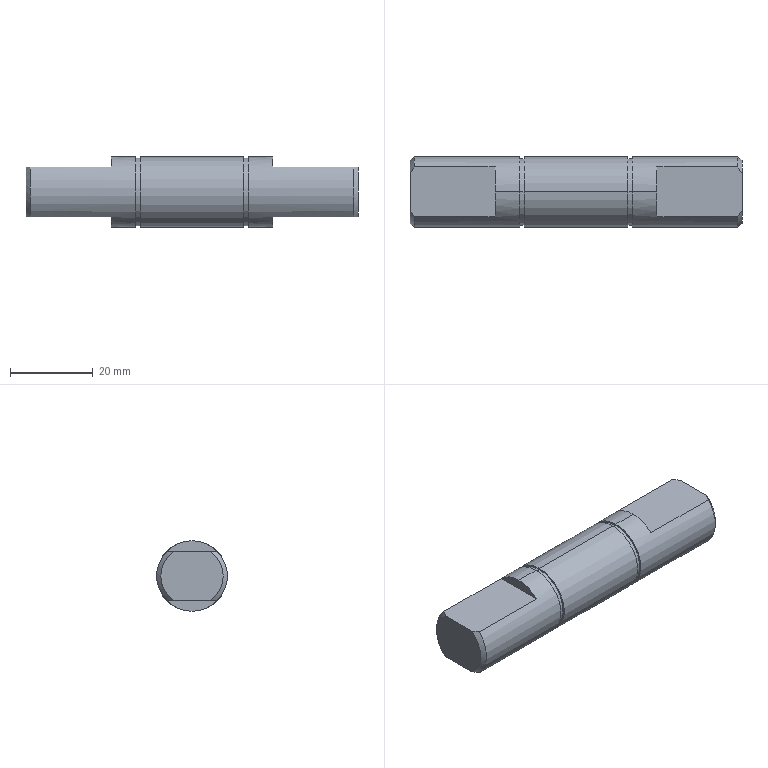Part | SolidWorks | features BaseBody 1 | 1 solid | 28 faces | box 80 x 17 x 17 mm | volume 16384 mm3 | plane 14 | cylinder 10 | cone 4 | commonest cylinder face diameters 17 x6 16.2 x4
STEP:
#1=CARTESIAN_POINT('',(12.5,0.,8.5));
#2=VERTEX_POINT('',#1);
#3=CARTESIAN_POINT('',(12.5,0.,-8.5));
#4=VERTEX_POINT('',#3);
#5=CARTESIAN_POINT('',(12.5,0.,0.));
#6=DIRECTION('',(-1.,0.,0.));
#7=DIRECTION('',(0.,0.,1.));
#8=AXIS2_PLACEMENT_3D('',#5,#6,#7);
#9=CIRCLE('',#8,8.5);
#10=EDGE_CURVE('',#2,#4,#9,.T.);
#11=ORIENTED_EDGE('',*,*,#10,.T.);
#12=CARTESIAN_POINT('',(-12.5,0.,-8.5));
#13=VERTEX_POINT('',#12);
#14=CARTESIAN_POINT('',(40.,0.,-8.5));
#15=DIRECTION('',(-1.,0.,0.));
#16=VECTOR('',#15,1000.);
#17=LINE('',#14,#16);
#18=EDGE_CURVE('',#4,#13,#17,.T.);
#19=ORIENTED_EDGE('',*,*,#18,.T.);
#20=CARTESIAN_POINT('',(-12.5,0.,8.5));
#21=VERTEX_POINT('',#20);
#22=CARTESIAN_POINT('',(-12.5,0.,0.));
#23=DIRECTION('',(1.,0.,0.));
#24=DIRECTION('',(0.,0.,1.));
#25=AXIS2_PLACEMENT_3D('',#22,#23,#24);
#26=CIRCLE('',#25,8.5);
#27=EDGE_CURVE('',#13,#21,#26,.T.);
#28=ORIENTED_EDGE('',*,*,#27,.T.);
#29=CARTESIAN_POINT('',(40.,0.,8.5));
#30=DIRECTION('',(-1.,0.,0.));
#31=VECTOR('',#30,1000.);
#32=LINE('',#29,#31);
#33=EDGE_CURVE('',#2,#21,#32,.T.);
#34=ORIENTED_EDGE('',*,*,#33,.F.);
#35=EDGE_LOOP('',(#11,#19,#28,#34));
#36=FACE_OUTER_BOUND('',#35,.T.);
#37=CARTESIAN_POINT('',(40.,0.,0.));
#38=DIRECTION('',(-1.,0.,0.));
#39=DIRECTION('',(0.,0.,1.));
#40=AXIS2_PLACEMENT_3D('',#37,#38,#39);
#41=CYLINDRICAL_SURFACE('',#40,8.5);
#42=ADVANCED_FACE('',(#36),#41,.T.);
#43=CARTESIAN_POINT('',(13.6,0.,8.1));
#44=VERTEX_POINT('',#43);
#45=CARTESIAN_POINT('',(13.6,0.,-8.1));
#46=VERTEX_POINT('',#45);
#47=CARTESIAN_POINT('',(13.6,0.,0.));
#48=DIRECTION('',(-1.,0.,0.));
#49=DIRECTION('',(0.,0.,1.));
#50=AXIS2_PLACEMENT_3D('',#47,#48,#49);
#51=CIRCLE('',#50,8.1);
#52=EDGE_CURVE('',#44,#46,#51,.T.);
#53=ORIENTED_EDGE('',*,*,#52,.T.);
#54=CARTESIAN_POINT('',(12.5,0.,-8.1));
#55=VERTEX_POINT('',#54);
#56=CARTESIAN_POINT('',(13.05,0.,-8.1));
#57=DIRECTION('',(-1.,0.,0.));
#58=VECTOR('',#57,1000.);
#59=LINE('',#56,#58);
#60=EDGE_CURVE('',#46,#55,#59,.T.);
#61=ORIENTED_EDGE('',*,*,#60,.T.);
#62=CARTESIAN_POINT('',(12.5,0.,8.1));
#63=VERTEX_POINT('',#62);
#64=CARTESIAN_POINT('',(12.5,0.,0.));
#65=DIRECTION('',(1.,0.,0.));
#66=DIRECTION('',(0.,0.,1.));
#67=AXIS2_PLACEMENT_3D('',#64,#65,#66);
#68=CIRCLE('',#67,8.1);
#69=EDGE_CURVE('',#55,#63,#68,.T.);
#70=ORIENTED_EDGE('',*,*,#69,.T.);
#71=CARTESIAN_POINT('',(13.05,0.,8.1));
#72=DIRECTION('',(-1.,0.,0.));
#73=VECTOR('',#72,1000.);
#74=LINE('',#71,#73);
#75=EDGE_CURVE('',#44,#63,#74,.T.);
#76=ORIENTED_EDGE('',*,*,#75,.F.);
#77=EDGE_LOOP('',(#53,#61,#70,#76));
#78=FACE_OUTER_BOUND('',#77,.T.);
#79=CARTESIAN_POINT('',(13.05,0.,0.));
#80=DIRECTION('',(-1.,0.,0.));
#81=DIRECTION('',(0.,0.,1.));
#82=AXIS2_PLACEMENT_3D('',#79,#80,#81);
#83=CYLINDRICAL_SURFACE('',#82,8.1);
#84=ADVANCED_FACE('',(#78),#83,.T.);
#85=CARTESIAN_POINT('',(-13.6,0.,-8.1));
#86=VERTEX_POINT('',#85);
#87=CARTESIAN_POINT('',(-13.6,0.,8.1));
#88=VERTEX_POINT('',#87);
#89=CARTESIAN_POINT('',(-13.6,0.,0.));
#90=DIRECTION('',(1.,0.,0.));
#91=DIRECTION('',(0.,0.,-1.));
#92=AXIS2_PLACEMENT_3D('',#89,#90,#91);
#93=CIRCLE('',#92,8.1);
#94=EDGE_CURVE('',#86,#88,#93,.T.);
#95=ORIENTED_EDGE('',*,*,#94,.T.);
#96=CARTESIAN_POINT('',(-12.5,0.,8.1));
#97=VERTEX_POINT('',#96);
#98=CARTESIAN_POINT('',(-13.05,0.,8.1));
#99=DIRECTION('',(1.,0.,0.));
#100=VECTOR('',#99,1000.);
#101=LINE('',#98,#100);
#102=EDGE_CURVE('',#88,#97,#101,.T.);
#103=ORIENTED_EDGE('',*,*,#102,.T.);
#104=CARTESIAN_POINT('',(-12.5,0.,-8.1));
#105=VERTEX_POINT('',#104);
#106=CARTESIAN_POINT('',(-12.5,0.,0.));
#107=DIRECTION('',(-1.,0.,0.));
#108=DIRECTION('',(0.,0.,-1.));
#109=AXIS2_PLACEMENT_3D('',#106,#107,#108);
#110=CIRCLE('',#109,8.1);
#111=EDGE_CURVE('',#97,#105,#110,.T.);
#112=ORIENTED_EDGE('',*,*,#111,.T.);
#113=CARTESIAN_POINT('',(-13.05,0.,-8.1));
#114=DIRECTION('',(1.,0.,0.));
#115=VECTOR('',#114,1000.);
#116=LINE('',#113,#115);
#117=EDGE_CURVE('',#86,#105,#116,.T.);
#118=ORIENTED_EDGE('',*,*,#117,.F.);
#119=EDGE_LOOP('',(#95,#103,#112,#118));
#120=FACE_OUTER_BOUND('',#119,.T.);
#121=CARTESIAN_POINT('',(-13.05,0.,0.));
#122=DIRECTION('',(1.,0.,0.));
#123=DIRECTION('',(0.,0.,-1.));
#124=AXIS2_PLACEMENT_3D('',#121,#122,#123);
#125=CYLINDRICAL_SURFACE('',#124,8.1);
#126=ADVANCED_FACE('',(#120),#125,.T.);
#127=CARTESIAN_POINT('',(19.5,6.021,-6.));
#128=VERTEX_POINT('',#127);
#129=CARTESIAN_POINT('',(19.5,0.,-8.5));
#130=VERTEX_POINT('',#129);
#131=CARTESIAN_POINT('',(19.5,0.,0.));
#132=DIRECTION('',(-1.,0.,0.));
#133=DIRECTION('',(0.,0.,1.));
#134=AXIS2_PLACEMENT_3D('',#131,#132,#133);
#135=CIRCLE('',#134,8.5);
#136=EDGE_CURVE('',#128,#130,#135,.T.);
#137=ORIENTED_EDGE('',*,*,#136,.T.);
#138=CARTESIAN_POINT('',(13.6,0.,-8.5));
#139=VERTEX_POINT('',#138);
#140=CARTESIAN_POINT('',(40.,0.,-8.5));
#141=DIRECTION('',(-1.,0.,0.));
#142=VECTOR('',#141,1000.);
#143=LINE('',#140,#142);
#144=EDGE_CURVE('',#130,#139,#143,.T.);
#145=ORIENTED_EDGE('',*,*,#144,.T.);
#146=CARTESIAN_POINT('',(13.6,0.,8.5));
#147=VERTEX_POINT('',#146);
#148=CARTESIAN_POINT('',(13.6,0.,0.));
#149=DIRECTION('',(-1.,0.,0.));
#150=DIRECTION('',(0.,0.,1.));
#151=AXIS2_PLACEMENT_3D('',#148,#149,#150);
#152=CIRCLE('',#151,8.5);
#153=EDGE_CURVE('',#147,#139,#152,.T.);
#154=ORIENTED_EDGE('',*,*,#153,.F.);
#155=CARTESIAN_POINT('',(19.5,0.,8.5));
#156=VERTEX_POINT('',#155);
#157=CARTESIAN_POINT('',(40.,0.,8.5));
#158=DIRECTION('',(-1.,0.,0.));
#159=VECTOR('',#158,1000.);
#160=LINE('',#157,#159);
#161=EDGE_CURVE('',#156,#147,#160,.T.);
#162=ORIENTED_EDGE('',*,*,#161,.F.);
#163=CARTESIAN_POINT('',(19.5,6.021,6.));
#164=VERTEX_POINT('',#163);
#165=CARTESIAN_POINT('',(19.5,0.,0.));
#166=DIRECTION('',(-1.,0.,0.));
#167=DIRECTION('',(0.,0.,1.));
#168=AXIS2_PLACEMENT_3D('',#165,#166,#167);
#169=CIRCLE('',#168,8.5);
#170=EDGE_CURVE('',#156,#164,#169,.T.);
#171=ORIENTED_EDGE('',*,*,#170,.T.);
#172=CARTESIAN_POINT('',(39.,6.021,6.));
#173=VERTEX_POINT('',#172);
#174=CARTESIAN_POINT('',(40.,6.021,6.));
#175=DIRECTION('',(1.,0.,0.));
#176=VECTOR('',#175,1000.);
#177=LINE('',#174,#176);
#178=EDGE_CURVE('',#164,#173,#177,.T.);
#179=ORIENTED_EDGE('',*,*,#178,.T.);
#180=CARTESIAN_POINT('',(39.,6.021,-6.));
#181=VERTEX_POINT('',#180);
#182=CARTESIAN_POINT('',(39.,0.,0.));
#183=DIRECTION('',(-1.,0.,0.));
#184=DIRECTION('',(0.,0.,1.));
#185=AXIS2_PLACEMENT_3D('',#182,#183,#184);
#186=CIRCLE('',#185,8.5);
#187=EDGE_CURVE('',#173,#181,#186,.T.);
#188=ORIENTED_EDGE('',*,*,#187,.T.);
#189=CARTESIAN_POINT('',(40.,6.021,-6.));
#190=DIRECTION('',(-1.,0.,0.));
#191=VECTOR('',#190,1000.);
#192=LINE('',#189,#191);
#193=EDGE_CURVE('',#181,#128,#192,.T.);
#194=ORIENTED_EDGE('',*,*,#193,.T.);
#195=EDGE_LOOP('',(#137,#145,#154,#162,#171,#179,#188,#194));
#196=FACE_OUTER_BOUND('',#195,.T.);
#197=CARTESIAN_POINT('',(40.,0.,0.));
#198=DIRECTION('',(-1.,0.,0.));
#199=DIRECTION('',(0.,0.,1.));
#200=AXIS2_PLACEMENT_3D('',#197,#198,#199);
#201=CYLINDRICAL_SURFACE('',#200,8.5);
#202=ADVANCED_FACE('',(#196),#201,.T.);
#203=CARTESIAN_POINT('',(-13.6,0.,-8.5));
#204=VERTEX_POINT('',#203);
#205=CARTESIAN_POINT('',(-13.6,0.,8.5));
#206=VERTEX_POINT('',#205);
#207=CARTESIAN_POINT('',(-13.6,0.,0.));
#208=DIRECTION('',(1.,0.,0.));
#209=DIRECTION('',(0.,0.,1.));
#210=AXIS2_PLACEMENT_3D('',#207,#208,#209);
#211=CIRCLE('',#210,8.5);
#212=EDGE_CURVE('',#204,#206,#211,.T.);
#213=ORIENTED_EDGE('',*,*,#212,.F.);
#214=CARTESIAN_POINT('',(-19.5,0.,-8.5));
#215=VERTEX_POINT('',#214);
#216=CARTESIAN_POINT('',(40.,0.,-8.5));
#217=DIRECTION('',(-1.,0.,0.));
#218=VECTOR('',#217,1000.);
#219=LINE('',#216,#218);
#220=EDGE_CURVE('',#204,#215,#219,.T.);
#221=ORIENTED_EDGE('',*,*,#220,.T.);
#222=CARTESIAN_POINT('',(-19.5,6.021,-6.));
#223=VERTEX_POINT('',#222);
#224=CARTESIAN_POINT('',(-19.5,0.,0.));
#225=DIRECTION('',(1.,0.,0.));
#226=DIRECTION('',(0.,0.,1.));
#227=AXIS2_PLACEMENT_3D('',#224,#225,#226);
#228=CIRCLE('',#227,8.5);
#229=EDGE_CURVE('',#215,#223,#228,.T.);
#230=ORIENTED_EDGE('',*,*,#229,.T.);
#231=CARTESIAN_POINT('',(-39.,6.021,-6.));
#232=VERTEX_POINT('',#231);
#233=CARTESIAN_POINT('',(40.,6.021,-6.));
#234=DIRECTION('',(-1.,0.,0.));
#235=VECTOR('',#234,1000.);
#236=LINE('',#233,#235);
#237=EDGE_CURVE('',#223,#232,#236,.T.);
#238=ORIENTED_EDGE('',*,*,#237,.T.);
#239=CARTESIAN_POINT('',(-39.,6.021,6.));
#240=VERTEX_POINT('',#239);
#241=CARTESIAN_POINT('',(-39.,0.,0.));
#242=DIRECTION('',(1.,0.,0.));
#243=DIRECTION('',(0.,0.,1.));
#244=AXIS2_PLACEMENT_3D('',#241,#242,#243);
#245=CIRCLE('',#244,8.5);
#246=EDGE_CURVE('',#232,#240,#245,.T.);
#247=ORIENTED_EDGE('',*,*,#246,.T.);
#248=CARTESIAN_POINT('',(-19.5,6.021,6.));
#249=VERTEX_POINT('',#248);
#250=CARTESIAN_POINT('',(40.,6.021,6.));
#251=DIRECTION('',(1.,0.,0.));
#252=VECTOR('',#251,1000.);
#253=LINE('',#250,#252);
#254=EDGE_CURVE('',#240,#249,#253,.T.);
#255=ORIENTED_EDGE('',*,*,#254,.T.);
#256=CARTESIAN_POINT('',(-19.5,0.,8.5));
#257=VERTEX_POINT('',#256);
#258=CARTESIAN_POINT('',(-19.5,0.,0.));
#259=DIRECTION('',(1.,0.,0.));
#260=DIRECTION('',(0.,0.,1.));
#261=AXIS2_PLACEMENT_3D('',#258,#259,#260);
#262=CIRCLE('',#261,8.5);
#263=EDGE_CURVE('',#249,#257,#262,.T.);
#264=ORIENTED_EDGE('',*,*,#263,.T.);
#265=CARTESIAN_POINT('',(40.,0.,8.5));
#266=DIRECTION('',(-1.,0.,0.));
#267=VECTOR('',#266,1000.);
#268=LINE('',#265,#267);
#269=EDGE_CURVE('',#206,#257,#268,.T.);
#270=ORIENTED_EDGE('',*,*,#269,.F.);
#271=EDGE_LOOP('',(#213,#221,#230,#238,#247,#255,#264,#270));
#272=FACE_OUTER_BOUND('',#271,.T.);
#273=CARTESIAN_POINT('',(40.,0.,0.));
#274=DIRECTION('',(-1.,0.,0.));
#275=DIRECTION('',(0.,0.,1.));
#276=AXIS2_PLACEMENT_3D('',#273,#274,#275);
#277=CYLINDRICAL_SURFACE('',#276,8.5);
#278=ADVANCED_FACE('',(#272),#277,.T.);
#279=ORIENTED_EDGE('',*,*,#18,.F.);
#280=CARTESIAN_POINT('',(12.5,0.,0.));
#281=DIRECTION('',(-1.,0.,0.));
#282=DIRECTION('',(0.,0.,1.));
#283=AXIS2_PLACEMENT_3D('',#280,#281,#282);
#284=CIRCLE('',#283,8.5);
#285=EDGE_CURVE('',#4,#2,#284,.T.);
#286=ORIENTED_EDGE('',*,*,#285,.T.);
#287=ORIENTED_EDGE('',*,*,#33,.T.);
#288=CARTESIAN_POINT('',(-12.5,0.,0.));
#289=DIRECTION('',(1.,0.,0.));
#290=DIRECTION('',(0.,0.,1.));
#291=AXIS2_PLACEMENT_3D('',#288,#289,#290);
#292=CIRCLE('',#291,8.5);
#293=EDGE_CURVE('',#21,#13,#292,.T.);
#294=ORIENTED_EDGE('',*,*,#293,.T.);
#295=EDGE_LOOP('',(#279,#286,#287,#294));
#296=FACE_OUTER_BOUND('',#295,.T.);
#297=CARTESIAN_POINT('',(40.,0.,0.));
#298=DIRECTION('',(-1.,0.,0.));
#299=DIRECTION('',(0.,0.,1.));
#300=AXIS2_PLACEMENT_3D('',#297,#298,#299);
#301=CYLINDRICAL_SURFACE('',#300,8.5);
#302=ADVANCED_FACE('',(#296),#301,.T.);
#303=ORIENTED_EDGE('',*,*,#10,.F.);
#304=ORIENTED_EDGE('',*,*,#285,.F.);
#305=EDGE_LOOP('',(#303,#304));
#306=FACE_OUTER_BOUND('',#305,.T.);
#307=CARTESIAN_POINT('',(12.5,0.,0.));
#308=DIRECTION('',(1.,0.,0.));
#309=DIRECTION('',(0.,0.,1.));
#310=AXIS2_PLACEMENT_3D('',#307,#308,#309);
#311=CIRCLE('',#310,8.1);
#312=EDGE_CURVE('',#63,#55,#311,.T.);
#313=ORIENTED_EDGE('',*,*,#312,.F.);
#314=ORIENTED_EDGE('',*,*,#69,.F.);
#315=EDGE_LOOP('',(#313,#314));
#316=FACE_BOUND('',#315,.T.);
#317=CARTESIAN_POINT('',(12.5,0.,0.));
#318=DIRECTION('',(-1.,0.,0.));
#319=DIRECTION('',(0.,0.,1.));
#320=AXIS2_PLACEMENT_3D('',#317,#318,#319);
#321=PLANE('',#320);
#322=ADVANCED_FACE('',(#306,#316),#321,.F.);
#323=ORIENTED_EDGE('',*,*,#293,.F.);
#324=ORIENTED_EDGE('',*,*,#27,.F.);
#325=EDGE_LOOP('',(#323,#324));
#326=FACE_OUTER_BOUND('',#325,.T.);
#327=CARTESIAN_POINT('',(-12.5,0.,0.));
#328=DIRECTION('',(-1.,0.,0.));
#329=DIRECTION('',(0.,0.,-1.));
#330=AXIS2_PLACEMENT_3D('',#327,#328,#329);
#331=CIRCLE('',#330,8.1);
#332=EDGE_CURVE('',#105,#97,#331,.T.);
#333=ORIENTED_EDGE('',*,*,#332,.F.);
#334=ORIENTED_EDGE('',*,*,#111,.F.);
#335=EDGE_LOOP('',(#333,#334));
#336=FACE_BOUND('',#335,.T.);
#337=CARTESIAN_POINT('',(-12.5,0.,0.));
#338=DIRECTION('',(1.,0.,0.));
#339=DIRECTION('',(0.,0.,-1.));
#340=AXIS2_PLACEMENT_3D('',#337,#338,#339);
#341=PLANE('',#340);
#342=ADVANCED_FACE('',(#326,#336),#341,.F.);
#343=ORIENTED_EDGE('',*,*,#60,.F.);
#344=CARTESIAN_POINT('',(13.6,0.,0.));
#345=DIRECTION('',(-1.,0.,0.));
#346=DIRECTION('',(0.,0.,1.));
#347=AXIS2_PLACEMENT_3D('',#344,#345,#346);
#348=CIRCLE('',#347,8.1);
#349=EDGE_CURVE('',#46,#44,#348,.T.);
#350=ORIENTED_EDGE('',*,*,#349,.T.);
#351=ORIENTED_EDGE('',*,*,#75,.T.);
#352=ORIENTED_EDGE('',*,*,#312,.T.);
#353=EDGE_LOOP('',(#343,#350,#351,#352));
#354=FACE_OUTER_BOUND('',#353,.T.);
#355=CARTESIAN_POINT('',(13.05,0.,0.));
#356=DIRECTION('',(-1.,0.,0.));
#357=DIRECTION('',(0.,0.,1.));
#358=AXIS2_PLACEMENT_3D('',#355,#356,#357);
#359=CYLINDRICAL_SURFACE('',#358,8.1);
#360=ADVANCED_FACE('',(#354),#359,.T.);
#361=ORIENTED_EDGE('',*,*,#102,.F.);
#362=CARTESIAN_POINT('',(-13.6,0.,0.));
#363=DIRECTION('',(1.,0.,0.));
#364=DIRECTION('',(0.,0.,-1.));
#365=AXIS2_PLACEMENT_3D('',#362,#363,#364);
#366=CIRCLE('',#365,8.1);
#367=EDGE_CURVE('',#88,#86,#366,.T.);
#368=ORIENTED_EDGE('',*,*,#367,.T.);
#369=ORIENTED_EDGE('',*,*,#117,.T.);
#370=ORIENTED_EDGE('',*,*,#332,.T.);
#371=EDGE_LOOP('',(#361,#368,#369,#370));
#372=FACE_OUTER_BOUND('',#371,.T.);
#373=CARTESIAN_POINT('',(-13.05,0.,0.));
#374=DIRECTION('',(1.,0.,0.));
#375=DIRECTION('',(0.,0.,-1.));
#376=AXIS2_PLACEMENT_3D('',#373,#374,#375);
#377=CYLINDRICAL_SURFACE('',#376,8.1);
#378=ADVANCED_FACE('',(#372),#377,.T.);
#379=ORIENTED_EDGE('',*,*,#153,.T.);
#380=CARTESIAN_POINT('',(13.6,0.,0.));
#381=DIRECTION('',(-1.,0.,0.));
#382=DIRECTION('',(0.,0.,1.));
#383=AXIS2_PLACEMENT_3D('',#380,#381,#382);
#384=CIRCLE('',#383,8.5);
#385=EDGE_CURVE('',#139,#147,#384,.T.);
#386=ORIENTED_EDGE('',*,*,#385,.T.);
#387=EDGE_LOOP('',(#379,#386));
#388=FACE_OUTER_BOUND('',#387,.T.);
#389=ORIENTED_EDGE('',*,*,#52,.F.);
#390=ORIENTED_EDGE('',*,*,#349,.F.);
#391=EDGE_LOOP('',(#389,#390));
#392=FACE_BOUND('',#391,.T.);
#393=CARTESIAN_POINT('',(13.6,0.,0.));
#394=DIRECTION('',(-1.,0.,0.));
#395=DIRECTION('',(0.,0.,1.));
#396=AXIS2_PLACEMENT_3D('',#393,#394,#395);
#397=PLANE('',#396);
#398=ADVANCED_FACE('',(#388,#392),#397,.T.);
#399=CARTESIAN_POINT('',(-13.6,0.,0.));
#400=DIRECTION('',(1.,0.,0.));
#401=DIRECTION('',(0.,0.,1.));
#402=AXIS2_PLACEMENT_3D('',#399,#400,#401);
#403=CIRCLE('',#402,8.5);
#404=EDGE_CURVE('',#206,#204,#403,.T.);
#405=ORIENTED_EDGE('',*,*,#404,.T.);
#406=ORIENTED_EDGE('',*,*,#212,.T.);
#407=EDGE_LOOP('',(#405,#406));
#408=FACE_OUTER_BOUND('',#407,.T.);
#409=ORIENTED_EDGE('',*,*,#94,.F.);
#410=ORIENTED_EDGE('',*,*,#367,.F.);
#411=EDGE_LOOP('',(#409,#410));
#412=FACE_BOUND('',#411,.T.);
#413=CARTESIAN_POINT('',(-13.6,0.,0.));
#414=DIRECTION('',(1.,0.,0.));
#415=DIRECTION('',(0.,0.,-1.));
#416=AXIS2_PLACEMENT_3D('',#413,#414,#415);
#417=PLANE('',#416);
#418=ADVANCED_FACE('',(#408,#412),#417,.T.);
#419=ORIENTED_EDGE('',*,*,#144,.F.);
#420=CARTESIAN_POINT('',(19.5,-6.021,-6.));
#421=VERTEX_POINT('',#420);
#422=CARTESIAN_POINT('',(19.5,0.,0.));
#423=DIRECTION('',(-1.,0.,0.));
#424=DIRECTION('',(0.,0.,1.));
#425=AXIS2_PLACEMENT_3D('',#422,#423,#424);
#426=CIRCLE('',#425,8.5);
#427=EDGE_CURVE('',#130,#421,#426,.T.);
#428=ORIENTED_EDGE('',*,*,#427,.T.);
#429=CARTESIAN_POINT('',(39.,-6.021,-6.));
#430=VERTEX_POINT('',#429);
#431=CARTESIAN_POINT('',(40.,-6.021,-6.));
#432=DIRECTION('',(1.,0.,0.));
#433=VECTOR('',#432,1000.);
#434=LINE('',#431,#433);
#435=EDGE_CURVE('',#421,#430,#434,.T.);
#436=ORIENTED_EDGE('',*,*,#435,.T.);
#437=CARTESIAN_POINT('',(39.,-6.021,6.));
#438=VERTEX_POINT('',#437);
#439=CARTESIAN_POINT('',(39.,0.,0.));
#440=DIRECTION('',(-1.,0.,0.));
#441=DIRECTION('',(0.,0.,1.));
#442=AXIS2_PLACEMENT_3D('',#439,#440,#441);
#443=CIRCLE('',#442,8.5);
#444=EDGE_CURVE('',#430,#438,#443,.T.);
#445=ORIENTED_EDGE('',*,*,#444,.T.);
#446=CARTESIAN_POINT('',(19.5,-6.021,6.));
#447=VERTEX_POINT('',#446);
#448=CARTESIAN_POINT('',(40.,-6.021,6.));
#449=DIRECTION('',(-1.,0.,0.));
#450=VECTOR('',#449,1000.);
#451=LINE('',#448,#450);
#452=EDGE_CURVE('',#438,#447,#451,.T.);
#453=ORIENTED_EDGE('',*,*,#452,.T.);
#454=CARTESIAN_POINT('',(19.5,0.,0.));
#455=DIRECTION('',(-1.,0.,0.));
#456=DIRECTION('',(0.,0.,1.));
#457=AXIS2_PLACEMENT_3D('',#454,#455,#456);
#458=CIRCLE('',#457,8.5);
#459=EDGE_CURVE('',#447,#156,#458,.T.);
#460=ORIENTED_EDGE('',*,*,#459,.T.);
#461=ORIENTED_EDGE('',*,*,#161,.T.);
#462=ORIENTED_EDGE('',*,*,#385,.F.);
#463=EDGE_LOOP('',(#419,#428,#436,#445,#453,#460,#461,#462));
#464=FACE_OUTER_BOUND('',#463,.T.);
#465=CARTESIAN_POINT('',(40.,0.,0.));
#466=DIRECTION('',(-1.,0.,0.));
#467=DIRECTION('',(0.,0.,1.));
#468=AXIS2_PLACEMENT_3D('',#465,#466,#467);
#469=CYLINDRICAL_SURFACE('',#468,8.5);
#470=ADVANCED_FACE('',(#464),#469,.T.);
#471=ORIENTED_EDGE('',*,*,#220,.F.);
#472=ORIENTED_EDGE('',*,*,#404,.F.);
#473=ORIENTED_EDGE('',*,*,#269,.T.);
#474=CARTESIAN_POINT('',(-19.5,-6.021,6.));
#475=VERTEX_POINT('',#474);
#476=CARTESIAN_POINT('',(-19.5,0.,0.));
#477=DIRECTION('',(1.,0.,0.));
#478=DIRECTION('',(0.,0.,1.));
#479=AXIS2_PLACEMENT_3D('',#476,#477,#478);
#480=CIRCLE('',#479,8.5);
#481=EDGE_CURVE('',#257,#475,#480,.T.);
#482=ORIENTED_EDGE('',*,*,#481,.T.);
#483=CARTESIAN_POINT('',(-39.,-6.021,6.));
#484=VERTEX_POINT('',#483);
#485=CARTESIAN_POINT('',(40.,-6.021,6.));
#486=DIRECTION('',(-1.,0.,0.));
#487=VECTOR('',#486,1000.);
#488=LINE('',#485,#487);
#489=EDGE_CURVE('',#475,#484,#488,.T.);
#490=ORIENTED_EDGE('',*,*,#489,.T.);
#491=CARTESIAN_POINT('',(-39.,-6.021,-6.));
#492=VERTEX_POINT('',#491);
#493=CARTESIAN_POINT('',(-39.,0.,0.));
#494=DIRECTION('',(1.,0.,0.));
#495=DIRECTION('',(0.,0.,1.));
#496=AXIS2_PLACEMENT_3D('',#493,#494,#495);
#497=CIRCLE('',#496,8.5);
#498=EDGE_CURVE('',#484,#492,#497,.T.);
#499=ORIENTED_EDGE('',*,*,#498,.T.);
#500=CARTESIAN_POINT('',(-19.5,-6.021,-6.));
#501=VERTEX_POINT('',#500);
#502=CARTESIAN_POINT('',(40.,-6.021,-6.));
#503=DIRECTION('',(1.,0.,0.));
#504=VECTOR('',#503,1000.);
#505=LINE('',#502,#504);
#506=EDGE_CURVE('',#492,#501,#505,.T.);
#507=ORIENTED_EDGE('',*,*,#506,.T.);
#508=CARTESIAN_POINT('',(-19.5,0.,0.));
#509=DIRECTION('',(1.,0.,0.));
#510=DIRECTION('',(0.,0.,1.));
#511=AXIS2_PLACEMENT_3D('',#508,#509,#510);
#512=CIRCLE('',#511,8.5);
#513=EDGE_CURVE('',#501,#215,#512,.T.);
#514=ORIENTED_EDGE('',*,*,#513,.T.);
#515=EDGE_LOOP('',(#471,#472,#473,#482,#490,#499,#507,#514));
#516=FACE_OUTER_BOUND('',#515,.T.);
#517=CARTESIAN_POINT('',(40.,0.,0.));
#518=DIRECTION('',(-1.,0.,0.));
#519=DIRECTION('',(0.,0.,1.));
#520=AXIS2_PLACEMENT_3D('',#517,#518,#519);
#521=CYLINDRICAL_SURFACE('',#520,8.5);
#522=ADVANCED_FACE('',(#516),#521,.T.);
#523=ORIENTED_EDGE('',*,*,#459,.F.);
#524=CARTESIAN_POINT('',(19.5,21.5,6.));
#525=DIRECTION('',(0.,1.,0.));
#526=VECTOR('',#525,1000.);
#527=LINE('',#524,#526);
#528=EDGE_CURVE('',#447,#164,#527,.T.);
#529=ORIENTED_EDGE('',*,*,#528,.T.);
#530=ORIENTED_EDGE('',*,*,#170,.F.);
#531=EDGE_LOOP('',(#523,#529,#530));
#532=FACE_OUTER_BOUND('',#531,.T.);
#533=CARTESIAN_POINT('',(19.5,21.5,36.));
#534=DIRECTION('',(1.,0.,0.));
#535=DIRECTION('',(0.,1.,0.));
#536=AXIS2_PLACEMENT_3D('',#533,#534,#535);
#537=PLANE('',#536);
#538=ADVANCED_FACE('',(#532),#537,.T.);
#539=ORIENTED_EDGE('',*,*,#452,.F.);
#540=CARTESIAN_POINT('',(40.,-4.5,6.));
#541=VERTEX_POINT('',#540);
#542=CARTESIAN_POINT('',(39.,-6.021,6.));
#543=CARTESIAN_POINT('',(39.351,-5.525,6.));
#544=CARTESIAN_POINT('',(39.688,-5.021,6.));
#545=CARTESIAN_POINT('',(40.,-4.5,6.));
#546=B_SPLINE_CURVE_WITH_KNOTS('',3,(#542,#543,#544,#545),.UNSPECIFIED.,.F.,.F.,(4,4),(0.,0.00182),.UNSPECIFIED.);
#547=EDGE_CURVE('',#438,#541,#546,.T.);
#548=ORIENTED_EDGE('',*,*,#547,.T.);
#549=CARTESIAN_POINT('',(40.,4.5,6.));
#550=VERTEX_POINT('',#549);
#551=CARTESIAN_POINT('',(40.,21.5,6.));
#552=DIRECTION('',(0.,1.,0.));
#553=VECTOR('',#552,1000.);
#554=LINE('',#551,#553);
#555=EDGE_CURVE('',#541,#550,#554,.T.);
#556=ORIENTED_EDGE('',*,*,#555,.T.);
#557=CARTESIAN_POINT('',(40.,4.5,6.));
#558=CARTESIAN_POINT('',(39.688,5.021,6.));
#559=CARTESIAN_POINT('',(39.351,5.525,6.));
#560=CARTESIAN_POINT('',(39.,6.021,6.));
#561=B_SPLINE_CURVE_WITH_KNOTS('',3,(#557,#558,#559,#560),.UNSPECIFIED.,.F.,.F.,(4,4),(0.,0.00182),.UNSPECIFIED.);
#562=EDGE_CURVE('',#550,#173,#561,.T.);
#563=ORIENTED_EDGE('',*,*,#562,.T.);
#564=ORIENTED_EDGE('',*,*,#178,.F.);
#565=ORIENTED_EDGE('',*,*,#528,.F.);
#566=EDGE_LOOP('',(#539,#548,#556,#563,#564,#565));
#567=FACE_OUTER_BOUND('',#566,.T.);
#568=CARTESIAN_POINT('',(19.5,21.5,6.));
#569=DIRECTION('',(0.,0.,1.));
#570=DIRECTION('',(1.,0.,0.));
#571=AXIS2_PLACEMENT_3D('',#568,#569,#570);
#572=PLANE('',#571);
#573=ADVANCED_FACE('',(#567),#572,.T.);
#574=CARTESIAN_POINT('',(40.,-4.5,-6.));
#575=VERTEX_POINT('',#574);
#576=CARTESIAN_POINT('',(39.,-6.021,-6.));
#577=CARTESIAN_POINT('',(39.351,-5.525,-6.));
#578=CARTESIAN_POINT('',(39.688,-5.021,-6.));
#579=CARTESIAN_POINT('',(40.,-4.5,-6.));
#580=B_SPLINE_CURVE_WITH_KNOTS('',3,(#576,#577,#578,#579),.UNSPECIFIED.,.F.,.F.,(4,4),(0.,0.00182),.UNSPECIFIED.);
#581=EDGE_CURVE('',#430,#575,#580,.T.);
#582=ORIENTED_EDGE('',*,*,#581,.T.);
#583=CARTESIAN_POINT('',(40.,0.,0.));
#584=DIRECTION('',(-1.,0.,0.));
#585=DIRECTION('',(0.,0.,1.));
#586=AXIS2_PLACEMENT_3D('',#583,#584,#585);
#587=CIRCLE('',#586,7.5);
#588=EDGE_CURVE('',#575,#541,#587,.T.);
#589=ORIENTED_EDGE('',*,*,#588,.T.);
#590=ORIENTED_EDGE('',*,*,#547,.F.);
#591=ORIENTED_EDGE('',*,*,#444,.F.);
#592=EDGE_LOOP('',(#582,#589,#590,#591));
#593=FACE_OUTER_BOUND('',#592,.T.);
#594=CARTESIAN_POINT('',(39.,0.,0.));
#595=DIRECTION('',(-1.,0.,0.));
#596=DIRECTION('',(0.,0.,1.));
#597=AXIS2_PLACEMENT_3D('',#594,#595,#596);
#598=CONICAL_SURFACE('',#597,8.5,0.7854);
#599=ADVANCED_FACE('',(#593),#598,.T.);
#600=ORIENTED_EDGE('',*,*,#435,.F.);
#601=CARTESIAN_POINT('',(19.5,21.5,-6.));
#602=DIRECTION('',(0.,1.,0.));
#603=VECTOR('',#602,1000.);
#604=LINE('',#601,#603);
#605=EDGE_CURVE('',#421,#128,#604,.T.);
#606=ORIENTED_EDGE('',*,*,#605,.T.);
#607=ORIENTED_EDGE('',*,*,#193,.F.);
#608=CARTESIAN_POINT('',(40.,4.5,-6.));
#609=VERTEX_POINT('',#608);
#610=CARTESIAN_POINT('',(39.,6.021,-6.));
#611=CARTESIAN_POINT('',(39.351,5.525,-6.));
#612=CARTESIAN_POINT('',(39.688,5.021,-6.));
#613=CARTESIAN_POINT('',(40.,4.5,-6.));
#614=B_SPLINE_CURVE_WITH_KNOTS('',3,(#610,#611,#612,#613),.UNSPECIFIED.,.F.,.F.,(4,4),(0.,0.00182),.UNSPECIFIED.);
#615=EDGE_CURVE('',#181,#609,#614,.T.);
#616=ORIENTED_EDGE('',*,*,#615,.T.);
#617=CARTESIAN_POINT('',(40.,21.5,-6.));
#618=DIRECTION('',(0.,-1.,0.));
#619=VECTOR('',#618,1000.);
#620=LINE('',#617,#619);
#621=EDGE_CURVE('',#609,#575,#620,.T.);
#622=ORIENTED_EDGE('',*,*,#621,.T.);
#623=ORIENTED_EDGE('',*,*,#581,.F.);
#624=EDGE_LOOP('',(#600,#606,#607,#616,#622,#623));
#625=FACE_OUTER_BOUND('',#624,.T.);
#626=CARTESIAN_POINT('',(19.5,21.5,-6.));
#627=DIRECTION('',(0.,0.,-1.));
#628=DIRECTION('',(-1.,0.,0.));
#629=AXIS2_PLACEMENT_3D('',#626,#627,#628);
#630=PLANE('',#629);
#631=ADVANCED_FACE('',(#625),#630,.T.);
#632=ORIENTED_EDGE('',*,*,#136,.F.);
#633=ORIENTED_EDGE('',*,*,#605,.F.);
#634=ORIENTED_EDGE('',*,*,#427,.F.);
#635=EDGE_LOOP('',(#632,#633,#634));
#636=FACE_OUTER_BOUND('',#635,.T.);
#637=CARTESIAN_POINT('',(19.5,21.5,-36.));
#638=DIRECTION('',(1.,0.,0.));
#639=DIRECTION('',(0.,1.,0.));
#640=AXIS2_PLACEMENT_3D('',#637,#638,#639);
#641=PLANE('',#640);
#642=ADVANCED_FACE('',(#636),#641,.T.);
#643=ORIENTED_EDGE('',*,*,#562,.F.);
#644=CARTESIAN_POINT('',(40.,0.,0.));
#645=DIRECTION('',(-1.,0.,0.));
#646=DIRECTION('',(0.,0.,1.));
#647=AXIS2_PLACEMENT_3D('',#644,#645,#646);
#648=CIRCLE('',#647,7.5);
#649=EDGE_CURVE('',#550,#609,#648,.T.);
#650=ORIENTED_EDGE('',*,*,#649,.T.);
#651=ORIENTED_EDGE('',*,*,#615,.F.);
#652=ORIENTED_EDGE('',*,*,#187,.F.);
#653=EDGE_LOOP('',(#643,#650,#651,#652));
#654=FACE_OUTER_BOUND('',#653,.T.);
#655=CARTESIAN_POINT('',(39.,0.,0.));
#656=DIRECTION('',(-1.,0.,0.));
#657=DIRECTION('',(0.,0.,1.));
#658=AXIS2_PLACEMENT_3D('',#655,#656,#657);
#659=CONICAL_SURFACE('',#658,8.5,0.7854);
#660=ADVANCED_FACE('',(#654),#659,.T.);
#661=ORIENTED_EDGE('',*,*,#513,.F.);
#662=CARTESIAN_POINT('',(-19.5,21.5,-6.));
#663=DIRECTION('',(0.,1.,0.));
#664=VECTOR('',#663,1000.);
#665=LINE('',#662,#664);
#666=EDGE_CURVE('',#501,#223,#665,.T.);
#667=ORIENTED_EDGE('',*,*,#666,.T.);
#668=ORIENTED_EDGE('',*,*,#229,.F.);
#669=EDGE_LOOP('',(#661,#667,#668));
#670=FACE_OUTER_BOUND('',#669,.T.);
#671=CARTESIAN_POINT('',(-19.5,21.5,-36.));
#672=DIRECTION('',(-1.,0.,0.));
#673=DIRECTION('',(0.,-1.,0.));
#674=AXIS2_PLACEMENT_3D('',#671,#672,#673);
#675=PLANE('',#674);
#676=ADVANCED_FACE('',(#670),#675,.T.);
#677=ORIENTED_EDGE('',*,*,#506,.F.);
#678=CARTESIAN_POINT('',(-40.,-4.5,-6.));
#679=VERTEX_POINT('',#678);
#680=CARTESIAN_POINT('',(-39.,-6.021,-6.));
#681=CARTESIAN_POINT('',(-39.351,-5.525,-6.));
#682=CARTESIAN_POINT('',(-39.688,-5.021,-6.));
#683=CARTESIAN_POINT('',(-40.,-4.5,-6.));
#684=B_SPLINE_CURVE_WITH_KNOTS('',3,(#680,#681,#682,#683),.UNSPECIFIED.,.F.,.F.,(4,4),(0.,0.00182),.UNSPECIFIED.);
#685=EDGE_CURVE('',#492,#679,#684,.T.);
#686=ORIENTED_EDGE('',*,*,#685,.T.);
#687=CARTESIAN_POINT('',(-40.,4.5,-6.));
#688=VERTEX_POINT('',#687);
#689=CARTESIAN_POINT('',(-40.,21.5,-6.));
#690=DIRECTION('',(0.,1.,0.));
#691=VECTOR('',#690,1000.);
#692=LINE('',#689,#691);
#693=EDGE_CURVE('',#679,#688,#692,.T.);
#694=ORIENTED_EDGE('',*,*,#693,.T.);
#695=CARTESIAN_POINT('',(-40.,4.5,-6.));
#696=CARTESIAN_POINT('',(-39.688,5.021,-6.));
#697=CARTESIAN_POINT('',(-39.351,5.525,-6.));
#698=CARTESIAN_POINT('',(-39.,6.021,-6.));
#699=B_SPLINE_CURVE_WITH_KNOTS('',3,(#695,#696,#697,#698),.UNSPECIFIED.,.F.,.F.,(4,4),(0.,0.00182),.UNSPECIFIED.);
#700=EDGE_CURVE('',#688,#232,#699,.T.);
#701=ORIENTED_EDGE('',*,*,#700,.T.);
#702=ORIENTED_EDGE('',*,*,#237,.F.);
#703=ORIENTED_EDGE('',*,*,#666,.F.);
#704=EDGE_LOOP('',(#677,#686,#694,#701,#702,#703));
#705=FACE_OUTER_BOUND('',#704,.T.);
#706=CARTESIAN_POINT('',(-19.5,21.5,-6.));
#707=DIRECTION('',(0.,0.,-1.));
#708=DIRECTION('',(-1.,0.,0.));
#709=AXIS2_PLACEMENT_3D('',#706,#707,#708);
#710=PLANE('',#709);
#711=ADVANCED_FACE('',(#705),#710,.T.);
#712=ORIENTED_EDGE('',*,*,#685,.F.);
#713=ORIENTED_EDGE('',*,*,#498,.F.);
#714=CARTESIAN_POINT('',(-40.,-4.5,6.));
#715=VERTEX_POINT('',#714);
#716=CARTESIAN_POINT('',(-39.,-6.021,6.));
#717=CARTESIAN_POINT('',(-39.351,-5.525,6.));
#718=CARTESIAN_POINT('',(-39.688,-5.021,6.));
#719=CARTESIAN_POINT('',(-40.,-4.5,6.));
#720=B_SPLINE_CURVE_WITH_KNOTS('',3,(#716,#717,#718,#719),.UNSPECIFIED.,.F.,.F.,(4,4),(0.,0.00182),.UNSPECIFIED.);
#721=EDGE_CURVE('',#484,#715,#720,.T.);
#722=ORIENTED_EDGE('',*,*,#721,.T.);
#723=CARTESIAN_POINT('',(-40.,0.,0.));
#724=DIRECTION('',(1.,0.,0.));
#725=DIRECTION('',(0.,0.,-1.));
#726=AXIS2_PLACEMENT_3D('',#723,#724,#725);
#727=CIRCLE('',#726,7.5);
#728=EDGE_CURVE('',#715,#679,#727,.T.);
#729=ORIENTED_EDGE('',*,*,#728,.T.);
#730=EDGE_LOOP('',(#712,#713,#722,#729));
#731=FACE_OUTER_BOUND('',#730,.T.);
#732=CARTESIAN_POINT('',(-39.,0.,0.));
#733=DIRECTION('',(1.,0.,0.));
#734=DIRECTION('',(0.,0.,-1.));
#735=AXIS2_PLACEMENT_3D('',#732,#733,#734);
#736=CONICAL_SURFACE('',#735,8.5,0.7854);
#737=ADVANCED_FACE('',(#731),#736,.T.);
#738=ORIENTED_EDGE('',*,*,#489,.F.);
#739=CARTESIAN_POINT('',(-19.5,21.5,6.));
#740=DIRECTION('',(0.,1.,0.));
#741=VECTOR('',#740,1000.);
#742=LINE('',#739,#741);
#743=EDGE_CURVE('',#475,#249,#742,.T.);
#744=ORIENTED_EDGE('',*,*,#743,.T.);
#745=ORIENTED_EDGE('',*,*,#254,.F.);
#746=CARTESIAN_POINT('',(-40.,4.5,6.));
#747=VERTEX_POINT('',#746);
#748=CARTESIAN_POINT('',(-39.,6.021,6.));
#749=CARTESIAN_POINT('',(-39.351,5.525,6.));
#750=CARTESIAN_POINT('',(-39.688,5.021,6.));
#751=CARTESIAN_POINT('',(-40.,4.5,6.));
#752=B_SPLINE_CURVE_WITH_KNOTS('',3,(#748,#749,#750,#751),.UNSPECIFIED.,.F.,.F.,(4,4),(0.,0.00182),.UNSPECIFIED.);
#753=EDGE_CURVE('',#240,#747,#752,.T.);
#754=ORIENTED_EDGE('',*,*,#753,.T.);
#755=CARTESIAN_POINT('',(-40.,21.5,6.));
#756=DIRECTION('',(0.,-1.,0.));
#757=VECTOR('',#756,1000.);
#758=LINE('',#755,#757);
#759=EDGE_CURVE('',#747,#715,#758,.T.);
#760=ORIENTED_EDGE('',*,*,#759,.T.);
#761=ORIENTED_EDGE('',*,*,#721,.F.);
#762=EDGE_LOOP('',(#738,#744,#745,#754,#760,#761));
#763=FACE_OUTER_BOUND('',#762,.T.);
#764=CARTESIAN_POINT('',(-19.5,21.5,6.));
#765=DIRECTION('',(0.,0.,1.));
#766=DIRECTION('',(1.,0.,0.));
#767=AXIS2_PLACEMENT_3D('',#764,#765,#766);
#768=PLANE('',#767);
#769=ADVANCED_FACE('',(#763),#768,.T.);
#770=ORIENTED_EDGE('',*,*,#263,.F.);
#771=ORIENTED_EDGE('',*,*,#743,.F.);
#772=ORIENTED_EDGE('',*,*,#481,.F.);
#773=EDGE_LOOP('',(#770,#771,#772));
#774=FACE_OUTER_BOUND('',#773,.T.);
#775=CARTESIAN_POINT('',(-19.5,21.5,36.));
#776=DIRECTION('',(-1.,0.,0.));
#777=DIRECTION('',(0.,-1.,0.));
#778=AXIS2_PLACEMENT_3D('',#775,#776,#777);
#779=PLANE('',#778);
#780=ADVANCED_FACE('',(#774),#779,.T.);
#781=ORIENTED_EDGE('',*,*,#753,.F.);
#782=ORIENTED_EDGE('',*,*,#246,.F.);
#783=ORIENTED_EDGE('',*,*,#700,.F.);
#784=CARTESIAN_POINT('',(-40.,0.,0.));
#785=DIRECTION('',(1.,0.,0.));
#786=DIRECTION('',(0.,0.,-1.));
#787=AXIS2_PLACEMENT_3D('',#784,#785,#786);
#788=CIRCLE('',#787,7.5);
#789=EDGE_CURVE('',#688,#747,#788,.T.);
#790=ORIENTED_EDGE('',*,*,#789,.T.);
#791=EDGE_LOOP('',(#781,#782,#783,#790));
#792=FACE_OUTER_BOUND('',#791,.T.);
#793=CARTESIAN_POINT('',(-39.,0.,0.));
#794=DIRECTION('',(1.,0.,0.));
#795=DIRECTION('',(0.,0.,-1.));
#796=AXIS2_PLACEMENT_3D('',#793,#794,#795);
#797=CONICAL_SURFACE('',#796,8.5,0.7854);
#798=ADVANCED_FACE('',(#792),#797,.T.);
#799=ORIENTED_EDGE('',*,*,#555,.F.);
#800=ORIENTED_EDGE('',*,*,#588,.F.);
#801=ORIENTED_EDGE('',*,*,#621,.F.);
#802=ORIENTED_EDGE('',*,*,#649,.F.);
#803=EDGE_LOOP('',(#799,#800,#801,#802));
#804=FACE_OUTER_BOUND('',#803,.T.);
#805=CARTESIAN_POINT('',(40.,0.,0.));
#806=DIRECTION('',(1.,0.,0.));
#807=DIRECTION('',(0.,0.,-1.));
#808=AXIS2_PLACEMENT_3D('',#805,#806,#807);
#809=PLANE('',#808);
#810=ADVANCED_FACE('',(#804),#809,.T.);
#811=ORIENTED_EDGE('',*,*,#789,.F.);
#812=ORIENTED_EDGE('',*,*,#693,.F.);
#813=ORIENTED_EDGE('',*,*,#728,.F.);
#814=ORIENTED_EDGE('',*,*,#759,.F.);
#815=EDGE_LOOP('',(#811,#812,#813,#814));
#816=FACE_OUTER_BOUND('',#815,.T.);
#817=CARTESIAN_POINT('',(-40.,0.,0.));
#818=DIRECTION('',(1.,0.,0.));
#819=DIRECTION('',(0.,0.,-1.));
#820=AXIS2_PLACEMENT_3D('',#817,#818,#819);
#821=PLANE('',#820);
#822=ADVANCED_FACE('',(#816),#821,.F.);
#823=CLOSED_SHELL('',(#42,#84,#126,#202,#278,#302,#322,#342,#360,#378,#398,#418,#470,#522,#538,#573,#599,#631,#642,#660,#676,#711,#737,#769,#780,#798,#810,#822));
#824=MANIFOLD_SOLID_BREP('',#823);
#825=CARTESIAN_POINT('',(0.,0.,0.));
#826=DIRECTION('',(0.,0.,1.));
#827=DIRECTION('',(1.,0.,0.));
#828=AXIS2_PLACEMENT_3D('',#825,#826,#827);
#829=(LENGTH_UNIT()NAMED_UNIT(*)SI_UNIT(.MILLI.,.METRE.));
#830=UNCERTAINTY_MEASURE_WITH_UNIT(LENGTH_MEASURE(0.00001),#829,'','');
#831=(NAMED_UNIT(*)PLANE_ANGLE_UNIT()SI_UNIT($,.RADIAN.));
#832=(NAMED_UNIT(*)SI_UNIT($,.STERADIAN.)SOLID_ANGLE_UNIT());
#833=(GEOMETRIC_REPRESENTATION_CONTEXT(3)GLOBAL_UNCERTAINTY_ASSIGNED_CONTEXT((#830))GLOBAL_UNIT_ASSIGNED_CONTEXT((#829,#831,#832))REPRESENTATION_CONTEXT('',''));
#834=ADVANCED_BREP_SHAPE_REPRESENTATION('',(#824,#828),#833);